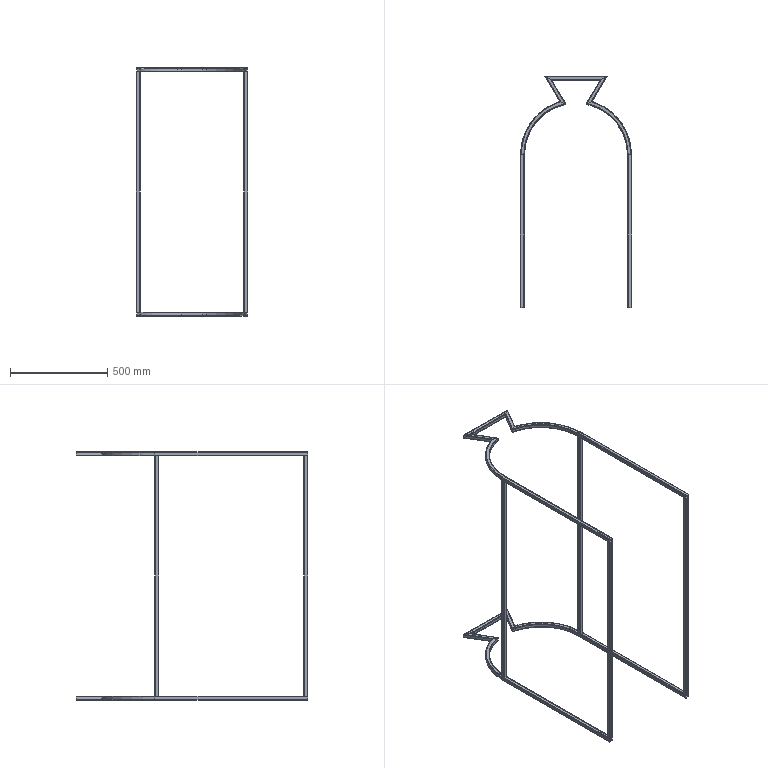Part | SolidWorks | 18 solids | 330 faces | box 574 x 1189 x 1276 mm | volume 911886 mm3 | plane 164 | cylinder 134 | spline 32 | commonest cylinder face diameters 3.6 x56 6 x56 530 x7 532.4 x7 567.6 x4 570 x4